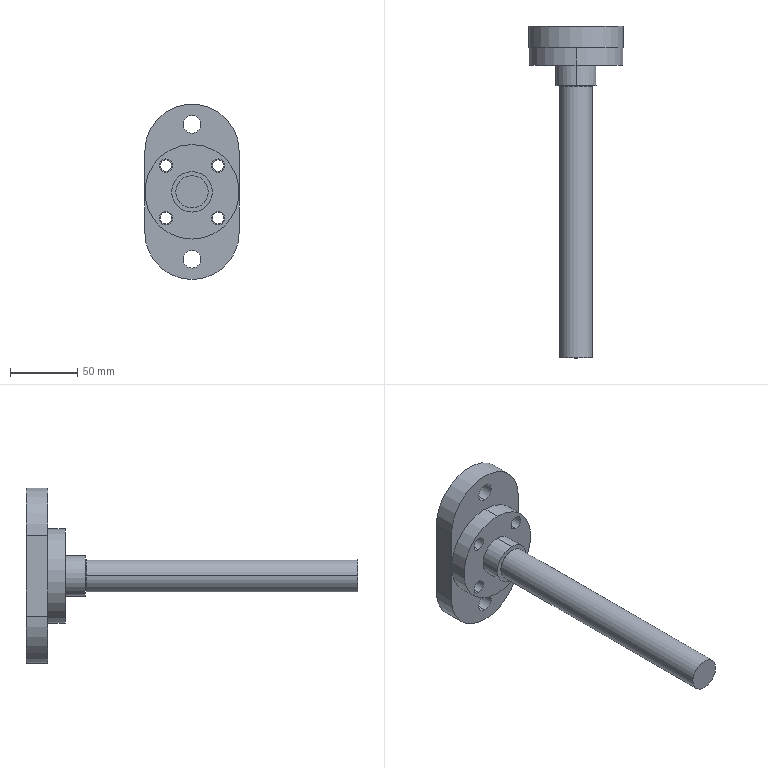Part | SolidWorks | features BaseBody 3 | 3 solids | 47 faces | box 70 x 246 x 130 mm | volume 268794 mm3 | cylinder 33 | plane 10 | cone 4 | commonest cylinder face diameters 8.5 x8 10 x8 70 x5 13 x4 16 x4 24 x2
STEP:
#1=CARTESIAN_POINT('',(-7.26,190.,0.));
#2=VERTEX_POINT('',#1);
#3=CARTESIAN_POINT('',(7.26,190.,0.));
#4=VERTEX_POINT('',#3);
#5=CARTESIAN_POINT('',(0.,190.,0.));
#6=DIRECTION('',(0.,1.,0.));
#7=DIRECTION('',(1.,0.,0.));
#8=AXIS2_PLACEMENT_3D('',#5,#6,#7);
#9=CIRCLE('',#8,7.26);
#10=EDGE_CURVE('',#2,#4,#9,.T.);
#11=ORIENTED_EDGE('',*,*,#10,.F.);
#12=CARTESIAN_POINT('',(-8.,189.26,0.));
#13=VERTEX_POINT('',#12);
#14=CARTESIAN_POINT('',(-7.26,190.,0.));
#15=DIRECTION('',(-0.7071,-0.7071,0.));
#16=VECTOR('',#15,1000.);
#17=LINE('',#14,#16);
#18=EDGE_CURVE('',#2,#13,#17,.T.);
#19=ORIENTED_EDGE('',*,*,#18,.T.);
#20=CARTESIAN_POINT('',(8.,189.26,0.));
#21=VERTEX_POINT('',#20);
#22=CARTESIAN_POINT('',(0.,189.26,0.));
#23=DIRECTION('',(0.,-1.,0.));
#24=DIRECTION('',(1.,0.,0.));
#25=AXIS2_PLACEMENT_3D('',#22,#23,#24);
#26=CIRCLE('',#25,8.);
#27=EDGE_CURVE('',#21,#13,#26,.T.);
#28=ORIENTED_EDGE('',*,*,#27,.F.);
#29=CARTESIAN_POINT('',(7.26,190.,0.));
#30=DIRECTION('',(0.7071,-0.7071,0.));
#31=VECTOR('',#30,1000.);
#32=LINE('',#29,#31);
#33=EDGE_CURVE('',#4,#21,#32,.T.);
#34=ORIENTED_EDGE('',*,*,#33,.F.);
#35=EDGE_LOOP('',(#11,#19,#28,#34));
#36=FACE_OUTER_BOUND('',#35,.T.);
#37=CARTESIAN_POINT('',(0.,190.,0.));
#38=DIRECTION('',(0.,-1.,0.));
#39=DIRECTION('',(1.,0.,0.));
#40=AXIS2_PLACEMENT_3D('',#37,#38,#39);
#41=CONICAL_SURFACE('',#40,7.26,0.7854);
#42=ADVANCED_FACE('',(#36),#41,.T.);
#43=CARTESIAN_POINT('',(-11.26,162.,0.));
#44=VERTEX_POINT('',#43);
#45=CARTESIAN_POINT('',(11.26,162.,0.));
#46=VERTEX_POINT('',#45);
#47=CARTESIAN_POINT('',(0.,162.,0.));
#48=DIRECTION('',(0.,1.,0.));
#49=DIRECTION('',(1.,0.,0.));
#50=AXIS2_PLACEMENT_3D('',#47,#48,#49);
#51=CIRCLE('',#50,11.26);
#52=EDGE_CURVE('',#44,#46,#51,.T.);
#53=ORIENTED_EDGE('',*,*,#52,.F.);
#54=CARTESIAN_POINT('',(-12.,161.26,0.));
#55=VERTEX_POINT('',#54);
#56=CARTESIAN_POINT('',(-11.26,162.,0.));
#57=DIRECTION('',(-0.7071,-0.7071,0.));
#58=VECTOR('',#57,1000.);
#59=LINE('',#56,#58);
#60=EDGE_CURVE('',#44,#55,#59,.T.);
#61=ORIENTED_EDGE('',*,*,#60,.T.);
#62=CARTESIAN_POINT('',(12.,161.26,0.));
#63=VERTEX_POINT('',#62);
#64=CARTESIAN_POINT('',(0.,161.26,0.));
#65=DIRECTION('',(0.,-1.,0.));
#66=DIRECTION('',(1.,0.,0.));
#67=AXIS2_PLACEMENT_3D('',#64,#65,#66);
#68=CIRCLE('',#67,12.);
#69=EDGE_CURVE('',#63,#55,#68,.T.);
#70=ORIENTED_EDGE('',*,*,#69,.F.);
#71=CARTESIAN_POINT('',(11.26,162.,0.));
#72=DIRECTION('',(0.7071,-0.7071,0.));
#73=VECTOR('',#72,1000.);
#74=LINE('',#71,#73);
#75=EDGE_CURVE('',#46,#63,#74,.T.);
#76=ORIENTED_EDGE('',*,*,#75,.F.);
#77=EDGE_LOOP('',(#53,#61,#70,#76));
#78=FACE_OUTER_BOUND('',#77,.T.);
#79=CARTESIAN_POINT('',(0.,162.,0.));
#80=DIRECTION('',(0.,-1.,0.));
#81=DIRECTION('',(1.,0.,0.));
#82=AXIS2_PLACEMENT_3D('',#79,#80,#81);
#83=CONICAL_SURFACE('',#82,11.26,0.7854);
#84=ADVANCED_FACE('',(#78),#83,.T.);
#85=CARTESIAN_POINT('',(-8.,162.,0.));
#86=VERTEX_POINT('',#85);
#87=CARTESIAN_POINT('',(8.,162.,0.));
#88=VERTEX_POINT('',#87);
#89=CARTESIAN_POINT('',(0.,162.,0.));
#90=DIRECTION('',(0.,1.,0.));
#91=DIRECTION('',(-1.,0.,0.));
#92=AXIS2_PLACEMENT_3D('',#89,#90,#91);
#93=CIRCLE('',#92,8.);
#94=EDGE_CURVE('',#86,#88,#93,.T.);
#95=ORIENTED_EDGE('',*,*,#94,.T.);
#96=CARTESIAN_POINT('',(8.,60.,0.));
#97=DIRECTION('',(0.,1.,0.));
#98=VECTOR('',#97,1000.);
#99=LINE('',#96,#98);
#100=EDGE_CURVE('',#88,#21,#99,.T.);
#101=ORIENTED_EDGE('',*,*,#100,.T.);
#102=ORIENTED_EDGE('',*,*,#27,.T.);
#103=CARTESIAN_POINT('',(-8.,60.,0.));
#104=DIRECTION('',(0.,1.,0.));
#105=VECTOR('',#104,1000.);
#106=LINE('',#103,#105);
#107=EDGE_CURVE('',#86,#13,#106,.T.);
#108=ORIENTED_EDGE('',*,*,#107,.F.);
#109=EDGE_LOOP('',(#95,#101,#102,#108));
#110=FACE_OUTER_BOUND('',#109,.T.);
#111=CARTESIAN_POINT('',(0.,60.,0.));
#112=DIRECTION('',(0.,1.,0.));
#113=DIRECTION('',(-1.,0.,0.));
#114=AXIS2_PLACEMENT_3D('',#111,#112,#113);
#115=CYLINDRICAL_SURFACE('',#114,8.);
#116=ADVANCED_FACE('',(#110),#115,.T.);
#117=CARTESIAN_POINT('',(-12.,-40.,0.));
#118=VERTEX_POINT('',#117);
#119=CARTESIAN_POINT('',(12.,-40.,0.));
#120=VERTEX_POINT('',#119);
#121=CARTESIAN_POINT('',(0.,-40.,0.));
#122=DIRECTION('',(0.,1.,0.));
#123=DIRECTION('',(-1.,0.,0.));
#124=AXIS2_PLACEMENT_3D('',#121,#122,#123);
#125=CIRCLE('',#124,12.);
#126=EDGE_CURVE('',#118,#120,#125,.T.);
#127=ORIENTED_EDGE('',*,*,#126,.T.);
#128=CARTESIAN_POINT('',(12.,60.,0.));
#129=DIRECTION('',(0.,1.,0.));
#130=VECTOR('',#129,1000.);
#131=LINE('',#128,#130);
#132=EDGE_CURVE('',#120,#63,#131,.T.);
#133=ORIENTED_EDGE('',*,*,#132,.T.);
#134=ORIENTED_EDGE('',*,*,#69,.T.);
#135=CARTESIAN_POINT('',(-12.,60.,0.));
#136=DIRECTION('',(0.,1.,0.));
#137=VECTOR('',#136,1000.);
#138=LINE('',#135,#137);
#139=EDGE_CURVE('',#118,#55,#138,.T.);
#140=ORIENTED_EDGE('',*,*,#139,.F.);
#141=EDGE_LOOP('',(#127,#133,#134,#140));
#142=FACE_OUTER_BOUND('',#141,.T.);
#143=CARTESIAN_POINT('',(0.,60.,0.));
#144=DIRECTION('',(0.,1.,0.));
#145=DIRECTION('',(-1.,0.,0.));
#146=AXIS2_PLACEMENT_3D('',#143,#144,#145);
#147=CYLINDRICAL_SURFACE('',#146,12.);
#148=ADVANCED_FACE('',(#142),#147,.T.);
#149=ORIENTED_EDGE('',*,*,#126,.F.);
#150=CARTESIAN_POINT('',(0.,-40.,0.));
#151=DIRECTION('',(0.,1.,0.));
#152=DIRECTION('',(-1.,0.,0.));
#153=AXIS2_PLACEMENT_3D('',#150,#151,#152);
#154=CIRCLE('',#153,12.);
#155=EDGE_CURVE('',#120,#118,#154,.T.);
#156=ORIENTED_EDGE('',*,*,#155,.F.);
#157=EDGE_LOOP('',(#149,#156));
#158=FACE_OUTER_BOUND('',#157,.T.);
#159=CARTESIAN_POINT('',(-12.,-40.,0.));
#160=DIRECTION('',(0.,1.,0.));
#161=DIRECTION('',(-1.,0.,0.));
#162=AXIS2_PLACEMENT_3D('',#159,#160,#161);
#163=PLANE('',#162);
#164=ADVANCED_FACE('',(#158),#163,.F.);
#165=ORIENTED_EDGE('',*,*,#132,.F.);
#166=ORIENTED_EDGE('',*,*,#155,.T.);
#167=ORIENTED_EDGE('',*,*,#139,.T.);
#168=CARTESIAN_POINT('',(0.,161.26,0.));
#169=DIRECTION('',(0.,-1.,0.));
#170=DIRECTION('',(1.,0.,0.));
#171=AXIS2_PLACEMENT_3D('',#168,#169,#170);
#172=CIRCLE('',#171,12.);
#173=EDGE_CURVE('',#55,#63,#172,.T.);
#174=ORIENTED_EDGE('',*,*,#173,.T.);
#175=EDGE_LOOP('',(#165,#166,#167,#174));
#176=FACE_OUTER_BOUND('',#175,.T.);
#177=CARTESIAN_POINT('',(0.,60.,0.));
#178=DIRECTION('',(0.,1.,0.));
#179=DIRECTION('',(-1.,0.,0.));
#180=AXIS2_PLACEMENT_3D('',#177,#178,#179);
#181=CYLINDRICAL_SURFACE('',#180,12.);
#182=ADVANCED_FACE('',(#176),#181,.T.);
#183=CARTESIAN_POINT('',(0.,162.,0.));
#184=DIRECTION('',(0.,1.,0.));
#185=DIRECTION('',(1.,0.,0.));
#186=AXIS2_PLACEMENT_3D('',#183,#184,#185);
#187=CIRCLE('',#186,11.26);
#188=EDGE_CURVE('',#46,#44,#187,.T.);
#189=ORIENTED_EDGE('',*,*,#188,.T.);
#190=ORIENTED_EDGE('',*,*,#52,.T.);
#191=EDGE_LOOP('',(#189,#190));
#192=FACE_OUTER_BOUND('',#191,.T.);
#193=ORIENTED_EDGE('',*,*,#94,.F.);
#194=CARTESIAN_POINT('',(0.,162.,0.));
#195=DIRECTION('',(0.,1.,0.));
#196=DIRECTION('',(-1.,0.,0.));
#197=AXIS2_PLACEMENT_3D('',#194,#195,#196);
#198=CIRCLE('',#197,8.);
#199=EDGE_CURVE('',#88,#86,#198,.T.);
#200=ORIENTED_EDGE('',*,*,#199,.F.);
#201=EDGE_LOOP('',(#193,#200));
#202=FACE_BOUND('',#201,.T.);
#203=CARTESIAN_POINT('',(-8.,162.,0.));
#204=DIRECTION('',(0.,-1.,0.));
#205=DIRECTION('',(1.,0.,0.));
#206=AXIS2_PLACEMENT_3D('',#203,#204,#205);
#207=PLANE('',#206);
#208=ADVANCED_FACE('',(#192,#202),#207,.F.);
#209=ORIENTED_EDGE('',*,*,#100,.F.);
#210=ORIENTED_EDGE('',*,*,#199,.T.);
#211=ORIENTED_EDGE('',*,*,#107,.T.);
#212=CARTESIAN_POINT('',(0.,189.26,0.));
#213=DIRECTION('',(0.,-1.,0.));
#214=DIRECTION('',(1.,0.,0.));
#215=AXIS2_PLACEMENT_3D('',#212,#213,#214);
#216=CIRCLE('',#215,8.);
#217=EDGE_CURVE('',#13,#21,#216,.T.);
#218=ORIENTED_EDGE('',*,*,#217,.T.);
#219=EDGE_LOOP('',(#209,#210,#211,#218));
#220=FACE_OUTER_BOUND('',#219,.T.);
#221=CARTESIAN_POINT('',(0.,60.,0.));
#222=DIRECTION('',(0.,1.,0.));
#223=DIRECTION('',(-1.,0.,0.));
#224=AXIS2_PLACEMENT_3D('',#221,#222,#223);
#225=CYLINDRICAL_SURFACE('',#224,8.);
#226=ADVANCED_FACE('',(#220),#225,.T.);
#227=CARTESIAN_POINT('',(0.,190.,0.));
#228=DIRECTION('',(0.,1.,0.));
#229=DIRECTION('',(1.,0.,0.));
#230=AXIS2_PLACEMENT_3D('',#227,#228,#229);
#231=CIRCLE('',#230,7.26);
#232=EDGE_CURVE('',#4,#2,#231,.T.);
#233=ORIENTED_EDGE('',*,*,#232,.T.);
#234=ORIENTED_EDGE('',*,*,#10,.T.);
#235=EDGE_LOOP('',(#233,#234));
#236=FACE_OUTER_BOUND('',#235,.T.);
#237=CARTESIAN_POINT('',(0.,190.,0.));
#238=DIRECTION('',(0.,-1.,0.));
#239=DIRECTION('',(1.,0.,0.));
#240=AXIS2_PLACEMENT_3D('',#237,#238,#239);
#241=PLANE('',#240);
#242=ADVANCED_FACE('',(#236),#241,.F.);
#243=ORIENTED_EDGE('',*,*,#60,.F.);
#244=ORIENTED_EDGE('',*,*,#188,.F.);
#245=ORIENTED_EDGE('',*,*,#75,.T.);
#246=ORIENTED_EDGE('',*,*,#173,.F.);
#247=EDGE_LOOP('',(#243,#244,#245,#246));
#248=FACE_OUTER_BOUND('',#247,.T.);
#249=CARTESIAN_POINT('',(0.,162.,0.));
#250=DIRECTION('',(0.,-1.,0.));
#251=DIRECTION('',(1.,0.,0.));
#252=AXIS2_PLACEMENT_3D('',#249,#250,#251);
#253=CONICAL_SURFACE('',#252,11.26,0.7854);
#254=ADVANCED_FACE('',(#248),#253,.T.);
#255=ORIENTED_EDGE('',*,*,#18,.F.);
#256=ORIENTED_EDGE('',*,*,#232,.F.);
#257=ORIENTED_EDGE('',*,*,#33,.T.);
#258=ORIENTED_EDGE('',*,*,#217,.F.);
#259=EDGE_LOOP('',(#255,#256,#257,#258));
#260=FACE_OUTER_BOUND('',#259,.T.);
#261=CARTESIAN_POINT('',(0.,190.,0.));
#262=DIRECTION('',(0.,-1.,0.));
#263=DIRECTION('',(1.,0.,0.));
#264=AXIS2_PLACEMENT_3D('',#261,#262,#263);
#265=CONICAL_SURFACE('',#264,7.26,0.7854);
#266=ADVANCED_FACE('',(#260),#265,.T.);
#267=CLOSED_SHELL('',(#42,#84,#116,#148,#164,#182,#208,#226,#242,#254,#266));
#268=MANIFOLD_SOLID_BREP('',#267);
#269=CARTESIAN_POINT('',(19.445,190.,-14.445));
#270=VERTEX_POINT('',#269);
#271=CARTESIAN_POINT('',(19.445,190.,-24.445));
#272=VERTEX_POINT('',#271);
#273=CARTESIAN_POINT('',(19.445,190.,-19.445));
#274=DIRECTION('',(0.,-1.,0.));
#275=DIRECTION('',(0.,0.,-1.));
#276=AXIS2_PLACEMENT_3D('',#273,#274,#275);
#277=CIRCLE('',#276,5.);
#278=EDGE_CURVE('',#270,#272,#277,.T.);
#279=ORIENTED_EDGE('',*,*,#278,.F.);
#280=CARTESIAN_POINT('',(19.445,177.,-14.445));
#281=VERTEX_POINT('',#280);
#282=CARTESIAN_POINT('',(19.445,177.,-14.445));
#283=DIRECTION('',(0.,-1.,0.));
#284=VECTOR('',#283,1000.);
#285=LINE('',#282,#284);
#286=EDGE_CURVE('',#270,#281,#285,.T.);
#287=ORIENTED_EDGE('',*,*,#286,.T.);
#288=CARTESIAN_POINT('',(19.445,177.,-24.445));
#289=VERTEX_POINT('',#288);
#290=CARTESIAN_POINT('',(19.445,177.,-19.445));
#291=DIRECTION('',(0.,-1.,0.));
#292=DIRECTION('',(0.,0.,-1.));
#293=AXIS2_PLACEMENT_3D('',#290,#291,#292);
#294=CIRCLE('',#293,5.);
#295=EDGE_CURVE('',#281,#289,#294,.T.);
#296=ORIENTED_EDGE('',*,*,#295,.T.);
#297=CARTESIAN_POINT('',(19.445,177.,-24.445));
#298=DIRECTION('',(0.,-1.,0.));
#299=VECTOR('',#298,1000.);
#300=LINE('',#297,#299);
#301=EDGE_CURVE('',#272,#289,#300,.T.);
#302=ORIENTED_EDGE('',*,*,#301,.F.);
#303=EDGE_LOOP('',(#279,#287,#296,#302));
#304=FACE_OUTER_BOUND('',#303,.T.);
#305=CARTESIAN_POINT('',(19.445,177.,-19.445));
#306=DIRECTION('',(0.,-1.,0.));
#307=DIRECTION('',(0.,0.,-1.));
#308=AXIS2_PLACEMENT_3D('',#305,#306,#307);
#309=CYLINDRICAL_SURFACE('',#308,5.);
#310=ADVANCED_FACE('',(#304),#309,.F.);
#311=CARTESIAN_POINT('',(-19.445,190.,-14.445));
#312=VERTEX_POINT('',#311);
#313=CARTESIAN_POINT('',(-19.445,190.,-24.445));
#314=VERTEX_POINT('',#313);
#315=CARTESIAN_POINT('',(-19.445,190.,-19.445));
#316=DIRECTION('',(0.,-1.,0.));
#317=DIRECTION('',(0.,0.,-1.));
#318=AXIS2_PLACEMENT_3D('',#315,#316,#317);
#319=CIRCLE('',#318,5.);
#320=EDGE_CURVE('',#312,#314,#319,.T.);
#321=ORIENTED_EDGE('',*,*,#320,.F.);
#322=CARTESIAN_POINT('',(-19.445,177.,-14.445));
#323=VERTEX_POINT('',#322);
#324=CARTESIAN_POINT('',(-19.445,177.,-14.445));
#325=DIRECTION('',(0.,-1.,0.));
#326=VECTOR('',#325,1000.);
#327=LINE('',#324,#326);
#328=EDGE_CURVE('',#312,#323,#327,.T.);
#329=ORIENTED_EDGE('',*,*,#328,.T.);
#330=CARTESIAN_POINT('',(-19.445,177.,-24.445));
#331=VERTEX_POINT('',#330);
#332=CARTESIAN_POINT('',(-19.445,177.,-19.445));
#333=DIRECTION('',(0.,-1.,0.));
#334=DIRECTION('',(0.,0.,-1.));
#335=AXIS2_PLACEMENT_3D('',#332,#333,#334);
#336=CIRCLE('',#335,5.);
#337=EDGE_CURVE('',#323,#331,#336,.T.);
#338=ORIENTED_EDGE('',*,*,#337,.T.);
#339=CARTESIAN_POINT('',(-19.445,177.,-24.445));
#340=DIRECTION('',(0.,-1.,0.));
#341=VECTOR('',#340,1000.);
#342=LINE('',#339,#341);
#343=EDGE_CURVE('',#314,#331,#342,.T.);
#344=ORIENTED_EDGE('',*,*,#343,.F.);
#345=EDGE_LOOP('',(#321,#329,#338,#344));
#346=FACE_OUTER_BOUND('',#345,.T.);
#347=CARTESIAN_POINT('',(-19.445,177.,-19.445));
#348=DIRECTION('',(0.,-1.,0.));
#349=DIRECTION('',(0.,0.,-1.));
#350=AXIS2_PLACEMENT_3D('',#347,#348,#349);
#351=CYLINDRICAL_SURFACE('',#350,5.);
#352=ADVANCED_FACE('',(#346),#351,.F.);
#353=CARTESIAN_POINT('',(-19.445,190.,24.445));
#354=VERTEX_POINT('',#353);
#355=CARTESIAN_POINT('',(-19.445,190.,14.445));
#356=VERTEX_POINT('',#355);
#357=CARTESIAN_POINT('',(-19.445,190.,19.445));
#358=DIRECTION('',(0.,-1.,0.));
#359=DIRECTION('',(0.,0.,-1.));
#360=AXIS2_PLACEMENT_3D('',#357,#358,#359);
#361=CIRCLE('',#360,5.);
#362=EDGE_CURVE('',#354,#356,#361,.T.);
#363=ORIENTED_EDGE('',*,*,#362,.F.);
#364=CARTESIAN_POINT('',(-19.445,177.,24.445));
#365=VERTEX_POINT('',#364);
#366=CARTESIAN_POINT('',(-19.445,177.,24.445));
#367=DIRECTION('',(0.,-1.,0.));
#368=VECTOR('',#367,1000.);
#369=LINE('',#366,#368);
#370=EDGE_CURVE('',#354,#365,#369,.T.);
#371=ORIENTED_EDGE('',*,*,#370,.T.);
#372=CARTESIAN_POINT('',(-19.445,177.,14.445));
#373=VERTEX_POINT('',#372);
#374=CARTESIAN_POINT('',(-19.445,177.,19.445));
#375=DIRECTION('',(0.,-1.,0.));
#376=DIRECTION('',(0.,0.,-1.));
#377=AXIS2_PLACEMENT_3D('',#374,#375,#376);
#378=CIRCLE('',#377,5.);
#379=EDGE_CURVE('',#365,#373,#378,.T.);
#380=ORIENTED_EDGE('',*,*,#379,.T.);
#381=CARTESIAN_POINT('',(-19.445,177.,14.445));
#382=DIRECTION('',(0.,-1.,0.));
#383=VECTOR('',#382,1000.);
#384=LINE('',#381,#383);
#385=EDGE_CURVE('',#356,#373,#384,.T.);
#386=ORIENTED_EDGE('',*,*,#385,.F.);
#387=EDGE_LOOP('',(#363,#371,#380,#386));
#388=FACE_OUTER_BOUND('',#387,.T.);
#389=CARTESIAN_POINT('',(-19.445,177.,19.445));
#390=DIRECTION('',(0.,-1.,0.));
#391=DIRECTION('',(0.,0.,-1.));
#392=AXIS2_PLACEMENT_3D('',#389,#390,#391);
#393=CYLINDRICAL_SURFACE('',#392,5.);
#394=ADVANCED_FACE('',(#388),#393,.F.);
#395=CARTESIAN_POINT('',(19.445,190.,24.445));
#396=VERTEX_POINT('',#395);
#397=CARTESIAN_POINT('',(19.445,190.,14.445));
#398=VERTEX_POINT('',#397);
#399=CARTESIAN_POINT('',(19.445,190.,19.445));
#400=DIRECTION('',(0.,-1.,0.));
#401=DIRECTION('',(0.,0.,-1.));
#402=AXIS2_PLACEMENT_3D('',#399,#400,#401);
#403=CIRCLE('',#402,5.);
#404=EDGE_CURVE('',#396,#398,#403,.T.);
#405=ORIENTED_EDGE('',*,*,#404,.F.);
#406=CARTESIAN_POINT('',(19.445,177.,24.445));
#407=VERTEX_POINT('',#406);
#408=CARTESIAN_POINT('',(19.445,177.,24.445));
#409=DIRECTION('',(0.,-1.,0.));
#410=VECTOR('',#409,1000.);
#411=LINE('',#408,#410);
#412=EDGE_CURVE('',#396,#407,#411,.T.);
#413=ORIENTED_EDGE('',*,*,#412,.T.);
#414=CARTESIAN_POINT('',(19.445,177.,14.445));
#415=VERTEX_POINT('',#414);
#416=CARTESIAN_POINT('',(19.445,177.,19.445));
#417=DIRECTION('',(0.,-1.,0.));
#418=DIRECTION('',(0.,0.,-1.));
#419=AXIS2_PLACEMENT_3D('',#416,#417,#418);
#420=CIRCLE('',#419,5.);
#421=EDGE_CURVE('',#407,#415,#420,.T.);
#422=ORIENTED_EDGE('',*,*,#421,.T.);
#423=CARTESIAN_POINT('',(19.445,177.,14.445));
#424=DIRECTION('',(0.,-1.,0.));
#425=VECTOR('',#424,1000.);
#426=LINE('',#423,#425);
#427=EDGE_CURVE('',#398,#415,#426,.T.);
#428=ORIENTED_EDGE('',*,*,#427,.F.);
#429=EDGE_LOOP('',(#405,#413,#422,#428));
#430=FACE_OUTER_BOUND('',#429,.T.);
#431=CARTESIAN_POINT('',(19.445,177.,19.445));
#432=DIRECTION('',(0.,-1.,0.));
#433=DIRECTION('',(0.,0.,-1.));
#434=AXIS2_PLACEMENT_3D('',#431,#432,#433);
#435=CYLINDRICAL_SURFACE('',#434,5.);
#436=ADVANCED_FACE('',(#430),#435,.F.);
#437=CARTESIAN_POINT('',(0.,177.,35.));
#438=VERTEX_POINT('',#437);
#439=CARTESIAN_POINT('',(0.,177.,-35.));
#440=VERTEX_POINT('',#439);
#441=CARTESIAN_POINT('',(0.,177.,0.));
#442=DIRECTION('',(0.,1.,0.));
#443=DIRECTION('',(0.,0.,1.));
#444=AXIS2_PLACEMENT_3D('',#441,#442,#443);
#445=CIRCLE('',#444,35.);
#446=EDGE_CURVE('',#438,#440,#445,.T.);
#447=ORIENTED_EDGE('',*,*,#446,.T.);
#448=CARTESIAN_POINT('',(0.,190.,-35.));
#449=VERTEX_POINT('',#448);
#450=CARTESIAN_POINT('',(0.,190.,-35.));
#451=DIRECTION('',(0.,1.,0.));
#452=VECTOR('',#451,1000.);
#453=LINE('',#450,#452);
#454=EDGE_CURVE('',#440,#449,#453,.T.);
#455=ORIENTED_EDGE('',*,*,#454,.T.);
#456=CARTESIAN_POINT('',(0.,190.,35.));
#457=VERTEX_POINT('',#456);
#458=CARTESIAN_POINT('',(0.,190.,0.));
#459=DIRECTION('',(0.,1.,0.));
#460=DIRECTION('',(0.,0.,1.));
#461=AXIS2_PLACEMENT_3D('',#458,#459,#460);
#462=CIRCLE('',#461,35.);
#463=EDGE_CURVE('',#457,#449,#462,.T.);
#464=ORIENTED_EDGE('',*,*,#463,.F.);
#465=CARTESIAN_POINT('',(0.,190.,35.));
#466=DIRECTION('',(0.,1.,0.));
#467=VECTOR('',#466,1000.);
#468=LINE('',#465,#467);
#469=EDGE_CURVE('',#438,#457,#468,.T.);
#470=ORIENTED_EDGE('',*,*,#469,.F.);
#471=EDGE_LOOP('',(#447,#455,#464,#470));
#472=FACE_OUTER_BOUND('',#471,.T.);
#473=CARTESIAN_POINT('',(0.,190.,0.));
#474=DIRECTION('',(0.,1.,0.));
#475=DIRECTION('',(0.,0.,1.));
#476=AXIS2_PLACEMENT_3D('',#473,#474,#475);
#477=CYLINDRICAL_SURFACE('',#476,35.);
#478=ADVANCED_FACE('',(#472),#477,.T.);
#479=CARTESIAN_POINT('',(0.,162.,15.));
#480=VERTEX_POINT('',#479);
#481=CARTESIAN_POINT('',(0.,162.,-15.));
#482=VERTEX_POINT('',#481);
#483=CARTESIAN_POINT('',(0.,162.,0.));
#484=DIRECTION('',(0.,1.,0.));
#485=DIRECTION('',(0.,0.,1.));
#486=AXIS2_PLACEMENT_3D('',#483,#484,#485);
#487=CIRCLE('',#486,15.);
#488=EDGE_CURVE('',#480,#482,#487,.T.);
#489=ORIENTED_EDGE('',*,*,#488,.T.);
#490=CARTESIAN_POINT('',(0.,177.,-15.));
#491=VERTEX_POINT('',#490);
#492=CARTESIAN_POINT('',(0.,190.,-15.));
#493=DIRECTION('',(0.,1.,0.));
#494=VECTOR('',#493,1000.);
#495=LINE('',#492,#494);
#496=EDGE_CURVE('',#482,#491,#495,.T.);
#497=ORIENTED_EDGE('',*,*,#496,.T.);
#498=CARTESIAN_POINT('',(0.,177.,15.));
#499=VERTEX_POINT('',#498);
#500=CARTESIAN_POINT('',(0.,177.,0.));
#501=DIRECTION('',(0.,1.,0.));
#502=DIRECTION('',(0.,0.,1.));
#503=AXIS2_PLACEMENT_3D('',#500,#501,#502);
#504=CIRCLE('',#503,15.);
#505=EDGE_CURVE('',#499,#491,#504,.T.);
#506=ORIENTED_EDGE('',*,*,#505,.F.);
#507=CARTESIAN_POINT('',(0.,190.,15.));
#508=DIRECTION('',(0.,1.,0.));
#509=VECTOR('',#508,1000.);
#510=LINE('',#507,#509);
#511=EDGE_CURVE('',#480,#499,#510,.T.);
#512=ORIENTED_EDGE('',*,*,#511,.F.);
#513=EDGE_LOOP('',(#489,#497,#506,#512));
#514=FACE_OUTER_BOUND('',#513,.T.);
#515=CARTESIAN_POINT('',(0.,190.,0.));
#516=DIRECTION('',(0.,1.,0.));
#517=DIRECTION('',(0.,0.,1.));
#518=AXIS2_PLACEMENT_3D('',#515,#516,#517);
#519=CYLINDRICAL_SURFACE('',#518,15.);
#520=ADVANCED_FACE('',(#514),#519,.T.);
#521=CARTESIAN_POINT('',(0.,162.,-8.));
#522=VERTEX_POINT('',#521);
#523=CARTESIAN_POINT('',(0.,162.,8.));
#524=VERTEX_POINT('',#523);
#525=CARTESIAN_POINT('',(0.,162.,0.));
#526=DIRECTION('',(0.,1.,0.));
#527=DIRECTION('',(0.,0.,1.));
#528=AXIS2_PLACEMENT_3D('',#525,#526,#527);
#529=CIRCLE('',#528,8.);
#530=EDGE_CURVE('',#522,#524,#529,.T.);
#531=ORIENTED_EDGE('',*,*,#530,.F.);
#532=CARTESIAN_POINT('',(0.,190.,-8.));
#533=VERTEX_POINT('',#532);
#534=CARTESIAN_POINT('',(0.,190.,-8.));
#535=DIRECTION('',(0.,1.,0.));
#536=VECTOR('',#535,1000.);
#537=LINE('',#534,#536);
#538=EDGE_CURVE('',#522,#533,#537,.T.);
#539=ORIENTED_EDGE('',*,*,#538,.T.);
#540=CARTESIAN_POINT('',(0.,190.,8.));
#541=VERTEX_POINT('',#540);
#542=CARTESIAN_POINT('',(0.,190.,0.));
#543=DIRECTION('',(0.,1.,0.));
#544=DIRECTION('',(0.,0.,1.));
#545=AXIS2_PLACEMENT_3D('',#542,#543,#544);
#546=CIRCLE('',#545,8.);
#547=EDGE_CURVE('',#533,#541,#546,.T.);
#548=ORIENTED_EDGE('',*,*,#547,.T.);
#549=CARTESIAN_POINT('',(0.,190.,8.));
#550=DIRECTION('',(0.,1.,0.));
#551=VECTOR('',#550,1000.);
#552=LINE('',#549,#551);
#553=EDGE_CURVE('',#524,#541,#552,.T.);
#554=ORIENTED_EDGE('',*,*,#553,.F.);
#555=EDGE_LOOP('',(#531,#539,#548,#554));
#556=FACE_OUTER_BOUND('',#555,.T.);
#557=CARTESIAN_POINT('',(0.,190.,0.));
#558=DIRECTION('',(0.,1.,0.));
#559=DIRECTION('',(0.,0.,1.));
#560=AXIS2_PLACEMENT_3D('',#557,#558,#559);
#561=CYLINDRICAL_SURFACE('',#560,8.);
#562=ADVANCED_FACE('',(#556),#561,.F.);
#563=ORIENTED_EDGE('',*,*,#538,.F.);
#564=CARTESIAN_POINT('',(0.,162.,0.));
#565=DIRECTION('',(0.,1.,0.));
#566=DIRECTION('',(0.,0.,1.));
#567=AXIS2_PLACEMENT_3D('',#564,#565,#566);
#568=CIRCLE('',#567,8.);
#569=EDGE_CURVE('',#524,#522,#568,.T.);
#570=ORIENTED_EDGE('',*,*,#569,.F.);
#571=ORIENTED_EDGE('',*,*,#553,.T.);
#572=CARTESIAN_POINT('',(0.,190.,0.));
#573=DIRECTION('',(0.,1.,0.));
#574=DIRECTION('',(0.,0.,1.));
#575=AXIS2_PLACEMENT_3D('',#572,#573,#574);
#576=CIRCLE('',#575,8.);
#577=EDGE_CURVE('',#541,#533,#576,.T.);
#578=ORIENTED_EDGE('',*,*,#577,.T.);
#579=EDGE_LOOP('',(#563,#570,#571,#578));
#580=FACE_OUTER_BOUND('',#579,.T.);
#581=CARTESIAN_POINT('',(0.,190.,0.));
#582=DIRECTION('',(0.,1.,0.));
#583=DIRECTION('',(0.,0.,1.));
#584=AXIS2_PLACEMENT_3D('',#581,#582,#583);
#585=CYLINDRICAL_SURFACE('',#584,8.);
#586=ADVANCED_FACE('',(#580),#585,.F.);
#587=ORIENTED_EDGE('',*,*,#488,.F.);
#588=CARTESIAN_POINT('',(0.,162.,0.));
#589=DIRECTION('',(0.,1.,0.));
#590=DIRECTION('',(0.,0.,1.));
#591=AXIS2_PLACEMENT_3D('',#588,#589,#590);
#592=CIRCLE('',#591,15.);
#593=EDGE_CURVE('',#482,#480,#592,.T.);
#594=ORIENTED_EDGE('',*,*,#593,.F.);
#595=EDGE_LOOP('',(#587,#594));
#596=FACE_OUTER_BOUND('',#595,.T.);
#597=ORIENTED_EDGE('',*,*,#569,.T.);
#598=ORIENTED_EDGE('',*,*,#530,.T.);
#599=EDGE_LOOP('',(#597,#598));
#600=FACE_BOUND('',#599,.T.);
#601=CARTESIAN_POINT('',(0.,162.,-8.));
#602=DIRECTION('',(0.,1.,0.));
#603=DIRECTION('',(0.,0.,1.));
#604=AXIS2_PLACEMENT_3D('',#601,#602,#603);
#605=PLANE('',#604);
#606=ADVANCED_FACE('',(#596,#600),#605,.F.);
#607=ORIENTED_EDGE('',*,*,#496,.F.);
#608=ORIENTED_EDGE('',*,*,#593,.T.);
#609=ORIENTED_EDGE('',*,*,#511,.T.);
#610=CARTESIAN_POINT('',(0.,177.,0.));
#611=DIRECTION('',(0.,1.,0.));
#612=DIRECTION('',(0.,0.,1.));
#613=AXIS2_PLACEMENT_3D('',#610,#611,#612);
#614=CIRCLE('',#613,15.);
#615=EDGE_CURVE('',#491,#499,#614,.T.);
#616=ORIENTED_EDGE('',*,*,#615,.F.);
#617=EDGE_LOOP('',(#607,#608,#609,#616));
#618=FACE_OUTER_BOUND('',#617,.T.);
#619=CARTESIAN_POINT('',(0.,190.,0.));
#620=DIRECTION('',(0.,1.,0.));
#621=DIRECTION('',(0.,0.,1.));
#622=AXIS2_PLACEMENT_3D('',#619,#620,#621);
#623=CYLINDRICAL_SURFACE('',#622,15.);
#624=ADVANCED_FACE('',(#618),#623,.T.);
#625=CARTESIAN_POINT('',(19.445,177.,-19.445));
#626=DIRECTION('',(0.,-1.,0.));
#627=DIRECTION('',(0.,0.,-1.));
#628=AXIS2_PLACEMENT_3D('',#625,#626,#627);
#629=CIRCLE('',#628,5.);
#630=EDGE_CURVE('',#289,#281,#629,.T.);
#631=ORIENTED_EDGE('',*,*,#630,.F.);
#632=ORIENTED_EDGE('',*,*,#295,.F.);
#633=EDGE_LOOP('',(#631,#632));
#634=FACE_BOUND('',#633,.T.);
#635=CARTESIAN_POINT('',(-19.445,177.,-19.445));
#636=DIRECTION('',(0.,-1.,0.));
#637=DIRECTION('',(0.,0.,-1.));
#638=AXIS2_PLACEMENT_3D('',#635,#636,#637);
#639=CIRCLE('',#638,5.);
#640=EDGE_CURVE('',#331,#323,#639,.T.);
#641=ORIENTED_EDGE('',*,*,#640,.F.);
#642=ORIENTED_EDGE('',*,*,#337,.F.);
#643=EDGE_LOOP('',(#641,#642));
#644=FACE_BOUND('',#643,.T.);
#645=CARTESIAN_POINT('',(-19.445,177.,19.445));
#646=DIRECTION('',(0.,-1.,0.));
#647=DIRECTION('',(0.,0.,-1.));
#648=AXIS2_PLACEMENT_3D('',#645,#646,#647);
#649=CIRCLE('',#648,5.);
#650=EDGE_CURVE('',#373,#365,#649,.T.);
#651=ORIENTED_EDGE('',*,*,#650,.F.);
#652=ORIENTED_EDGE('',*,*,#379,.F.);
#653=EDGE_LOOP('',(#651,#652));
#654=FACE_BOUND('',#653,.T.);
#655=CARTESIAN_POINT('',(19.445,177.,19.445));
#656=DIRECTION('',(0.,-1.,0.));
#657=DIRECTION('',(0.,0.,-1.));
#658=AXIS2_PLACEMENT_3D('',#655,#656,#657);
#659=CIRCLE('',#658,5.);
#660=EDGE_CURVE('',#415,#407,#659,.T.);
#661=ORIENTED_EDGE('',*,*,#660,.F.);
#662=ORIENTED_EDGE('',*,*,#421,.F.);
#663=EDGE_LOOP('',(#661,#662));
#664=FACE_BOUND('',#663,.T.);
#665=ORIENTED_EDGE('',*,*,#446,.F.);
#666=CARTESIAN_POINT('',(0.,177.,0.));
#667=DIRECTION('',(0.,1.,0.));
#668=DIRECTION('',(0.,0.,1.));
#669=AXIS2_PLACEMENT_3D('',#666,#667,#668);
#670=CIRCLE('',#669,35.);
#671=EDGE_CURVE('',#440,#438,#670,.T.);
#672=ORIENTED_EDGE('',*,*,#671,.F.);
#673=EDGE_LOOP('',(#665,#672));
#674=FACE_OUTER_BOUND('',#673,.T.);
#675=ORIENTED_EDGE('',*,*,#505,.T.);
#676=ORIENTED_EDGE('',*,*,#615,.T.);
#677=EDGE_LOOP('',(#675,#676));
#678=FACE_BOUND('',#677,.T.);
#679=CARTESIAN_POINT('',(0.,177.,-15.));
#680=DIRECTION('',(0.,1.,0.));
#681=DIRECTION('',(0.,0.,1.));
#682=AXIS2_PLACEMENT_3D('',#679,#680,#681);
#683=PLANE('',#682);
#684=ADVANCED_FACE('',(#634,#644,#654,#664,#674,#678),#683,.F.);
#685=ORIENTED_EDGE('',*,*,#454,.F.);
#686=ORIENTED_EDGE('',*,*,#671,.T.);
#687=ORIENTED_EDGE('',*,*,#469,.T.);
#688=CARTESIAN_POINT('',(0.,190.,0.));
#689=DIRECTION('',(0.,1.,0.));
#690=DIRECTION('',(0.,0.,1.));
#691=AXIS2_PLACEMENT_3D('',#688,#689,#690);
#692=CIRCLE('',#691,35.);
#693=EDGE_CURVE('',#449,#457,#692,.T.);
#694=ORIENTED_EDGE('',*,*,#693,.F.);
#695=EDGE_LOOP('',(#685,#686,#687,#694));
#696=FACE_OUTER_BOUND('',#695,.T.);
#697=CARTESIAN_POINT('',(0.,190.,0.));
#698=DIRECTION('',(0.,1.,0.));
#699=DIRECTION('',(0.,0.,1.));
#700=AXIS2_PLACEMENT_3D('',#697,#698,#699);
#701=CYLINDRICAL_SURFACE('',#700,35.);
#702=ADVANCED_FACE('',(#696),#701,.T.);
#703=CARTESIAN_POINT('',(19.445,190.,-19.445));
#704=DIRECTION('',(0.,-1.,0.));
#705=DIRECTION('',(0.,0.,-1.));
#706=AXIS2_PLACEMENT_3D('',#703,#704,#705);
#707=CIRCLE('',#706,5.);
#708=EDGE_CURVE('',#272,#270,#707,.T.);
#709=ORIENTED_EDGE('',*,*,#708,.T.);
#710=ORIENTED_EDGE('',*,*,#278,.T.);
#711=EDGE_LOOP('',(#709,#710));
#712=FACE_BOUND('',#711,.T.);
#713=CARTESIAN_POINT('',(-19.445,190.,-19.445));
#714=DIRECTION('',(0.,-1.,0.));
#715=DIRECTION('',(0.,0.,-1.));
#716=AXIS2_PLACEMENT_3D('',#713,#714,#715);
#717=CIRCLE('',#716,5.);
#718=EDGE_CURVE('',#314,#312,#717,.T.);
#719=ORIENTED_EDGE('',*,*,#718,.T.);
#720=ORIENTED_EDGE('',*,*,#320,.T.);
#721=EDGE_LOOP('',(#719,#720));
#722=FACE_BOUND('',#721,.T.);
#723=CARTESIAN_POINT('',(-19.445,190.,19.445));
#724=DIRECTION('',(0.,-1.,0.));
#725=DIRECTION('',(0.,0.,-1.));
#726=AXIS2_PLACEMENT_3D('',#723,#724,#725);
#727=CIRCLE('',#726,5.);
#728=EDGE_CURVE('',#356,#354,#727,.T.);
#729=ORIENTED_EDGE('',*,*,#728,.T.);
#730=ORIENTED_EDGE('',*,*,#362,.T.);
#731=EDGE_LOOP('',(#729,#730));
#732=FACE_BOUND('',#731,.T.);
#733=CARTESIAN_POINT('',(19.445,190.,19.445));
#734=DIRECTION('',(0.,-1.,0.));
#735=DIRECTION('',(0.,0.,-1.));
#736=AXIS2_PLACEMENT_3D('',#733,#734,#735);
#737=CIRCLE('',#736,5.);
#738=EDGE_CURVE('',#398,#396,#737,.T.);
#739=ORIENTED_EDGE('',*,*,#738,.T.);
#740=ORIENTED_EDGE('',*,*,#404,.T.);
#741=EDGE_LOOP('',(#739,#740));
#742=FACE_BOUND('',#741,.T.);
#743=ORIENTED_EDGE('',*,*,#577,.F.);
#744=ORIENTED_EDGE('',*,*,#547,.F.);
#745=EDGE_LOOP('',(#743,#744));
#746=FACE_BOUND('',#745,.T.);
#747=ORIENTED_EDGE('',*,*,#463,.T.);
#748=ORIENTED_EDGE('',*,*,#693,.T.);
#749=EDGE_LOOP('',(#747,#748));
#750=FACE_OUTER_BOUND('',#749,.T.);
#751=CARTESIAN_POINT('',(0.,190.,-35.));
#752=DIRECTION('',(0.,-1.,0.));
#753=DIRECTION('',(0.,0.,-1.));
#754=AXIS2_PLACEMENT_3D('',#751,#752,#753);
#755=PLANE('',#754);
#756=ADVANCED_FACE('',(#712,#722,#732,#742,#746,#750),#755,.F.);
#757=ORIENTED_EDGE('',*,*,#412,.F.);
#758=ORIENTED_EDGE('',*,*,#738,.F.);
#759=ORIENTED_EDGE('',*,*,#427,.T.);
#760=ORIENTED_EDGE('',*,*,#660,.T.);
#761=EDGE_LOOP('',(#757,#758,#759,#760));
#762=FACE_OUTER_BOUND('',#761,.T.);
#763=CARTESIAN_POINT('',(19.445,177.,19.445));
#764=DIRECTION('',(0.,-1.,0.));
#765=DIRECTION('',(0.,0.,-1.));
#766=AXIS2_PLACEMENT_3D('',#763,#764,#765);
#767=CYLINDRICAL_SURFACE('',#766,5.);
#768=ADVANCED_FACE('',(#762),#767,.F.);
#769=ORIENTED_EDGE('',*,*,#370,.F.);
#770=ORIENTED_EDGE('',*,*,#728,.F.);
#771=ORIENTED_EDGE('',*,*,#385,.T.);
#772=ORIENTED_EDGE('',*,*,#650,.T.);
#773=EDGE_LOOP('',(#769,#770,#771,#772));
#774=FACE_OUTER_BOUND('',#773,.T.);
#775=CARTESIAN_POINT('',(-19.445,177.,19.445));
#776=DIRECTION('',(0.,-1.,0.));
#777=DIRECTION('',(0.,0.,-1.));
#778=AXIS2_PLACEMENT_3D('',#775,#776,#777);
#779=CYLINDRICAL_SURFACE('',#778,5.);
#780=ADVANCED_FACE('',(#774),#779,.F.);
#781=ORIENTED_EDGE('',*,*,#328,.F.);
#782=ORIENTED_EDGE('',*,*,#718,.F.);
#783=ORIENTED_EDGE('',*,*,#343,.T.);
#784=ORIENTED_EDGE('',*,*,#640,.T.);
#785=EDGE_LOOP('',(#781,#782,#783,#784));
#786=FACE_OUTER_BOUND('',#785,.T.);
#787=CARTESIAN_POINT('',(-19.445,177.,-19.445));
#788=DIRECTION('',(0.,-1.,0.));
#789=DIRECTION('',(0.,0.,-1.));
#790=AXIS2_PLACEMENT_3D('',#787,#788,#789);
#791=CYLINDRICAL_SURFACE('',#790,5.);
#792=ADVANCED_FACE('',(#786),#791,.F.);
#793=ORIENTED_EDGE('',*,*,#286,.F.);
#794=ORIENTED_EDGE('',*,*,#708,.F.);
#795=ORIENTED_EDGE('',*,*,#301,.T.);
#796=ORIENTED_EDGE('',*,*,#630,.T.);
#797=EDGE_LOOP('',(#793,#794,#795,#796));
#798=FACE_OUTER_BOUND('',#797,.T.);
#799=CARTESIAN_POINT('',(19.445,177.,-19.445));
#800=DIRECTION('',(0.,-1.,0.));
#801=DIRECTION('',(0.,0.,-1.));
#802=AXIS2_PLACEMENT_3D('',#799,#800,#801);
#803=CYLINDRICAL_SURFACE('',#802,5.);
#804=ADVANCED_FACE('',(#798),#803,.F.);
#805=CLOSED_SHELL('',(#310,#352,#394,#436,#478,#520,#562,#586,#606,#624,#684,#702,#756,#768,#780,#792,#804));
#806=MANIFOLD_SOLID_BREP('',#805);
#807=CARTESIAN_POINT('',(0.,206.,56.5));
#808=VERTEX_POINT('',#807);
#809=CARTESIAN_POINT('',(0.,206.,43.5));
#810=VERTEX_POINT('',#809);
#811=CARTESIAN_POINT('',(0.,206.,50.));
#812=DIRECTION('',(0.,-1.,0.));
#813=DIRECTION('',(0.,0.,-1.));
#814=AXIS2_PLACEMENT_3D('',#811,#812,#813);
#815=CIRCLE('',#814,6.5);
#816=EDGE_CURVE('',#808,#810,#815,.T.);
#817=ORIENTED_EDGE('',*,*,#816,.F.);
#818=CARTESIAN_POINT('',(0.,190.,56.5));
#819=VERTEX_POINT('',#818);
#820=CARTESIAN_POINT('',(0.,206.,56.5));
#821=DIRECTION('',(0.,-1.,0.));
#822=VECTOR('',#821,1000.);
#823=LINE('',#820,#822);
#824=EDGE_CURVE('',#808,#819,#823,.T.);
#825=ORIENTED_EDGE('',*,*,#824,.T.);
#826=CARTESIAN_POINT('',(0.,190.,43.5));
#827=VERTEX_POINT('',#826);
#828=CARTESIAN_POINT('',(0.,190.,50.));
#829=DIRECTION('',(0.,-1.,0.));
#830=DIRECTION('',(0.,0.,-1.));
#831=AXIS2_PLACEMENT_3D('',#828,#829,#830);
#832=CIRCLE('',#831,6.5);
#833=EDGE_CURVE('',#819,#827,#832,.T.);
#834=ORIENTED_EDGE('',*,*,#833,.T.);
#835=CARTESIAN_POINT('',(0.,206.,43.5));
#836=DIRECTION('',(0.,-1.,0.));
#837=VECTOR('',#836,1000.);
#838=LINE('',#835,#837);
#839=EDGE_CURVE('',#810,#827,#838,.T.);
#840=ORIENTED_EDGE('',*,*,#839,.F.);
#841=EDGE_LOOP('',(#817,#825,#834,#840));
#842=FACE_OUTER_BOUND('',#841,.T.);
#843=CARTESIAN_POINT('',(0.,206.,50.));
#844=DIRECTION('',(0.,-1.,0.));
#845=DIRECTION('',(0.,0.,-1.));
#846=AXIS2_PLACEMENT_3D('',#843,#844,#845);
#847=CYLINDRICAL_SURFACE('',#846,6.5);
#848=ADVANCED_FACE('',(#842),#847,.F.);
#849=CARTESIAN_POINT('',(0.,206.,-43.5));
#850=VERTEX_POINT('',#849);
#851=CARTESIAN_POINT('',(0.,206.,-56.5));
#852=VERTEX_POINT('',#851);
#853=CARTESIAN_POINT('',(0.,206.,-50.));
#854=DIRECTION('',(0.,-1.,0.));
#855=DIRECTION('',(0.,0.,-1.));
#856=AXIS2_PLACEMENT_3D('',#853,#854,#855);
#857=CIRCLE('',#856,6.5);
#858=EDGE_CURVE('',#850,#852,#857,.T.);
#859=ORIENTED_EDGE('',*,*,#858,.F.);
#860=CARTESIAN_POINT('',(0.,190.,-43.5));
#861=VERTEX_POINT('',#860);
#862=CARTESIAN_POINT('',(0.,206.,-43.5));
#863=DIRECTION('',(0.,-1.,0.));
#864=VECTOR('',#863,1000.);
#865=LINE('',#862,#864);
#866=EDGE_CURVE('',#850,#861,#865,.T.);
#867=ORIENTED_EDGE('',*,*,#866,.T.);
#868=CARTESIAN_POINT('',(0.,190.,-56.5));
#869=VERTEX_POINT('',#868);
#870=CARTESIAN_POINT('',(0.,190.,-50.));
#871=DIRECTION('',(0.,-1.,0.));
#872=DIRECTION('',(0.,0.,-1.));
#873=AXIS2_PLACEMENT_3D('',#870,#871,#872);
#874=CIRCLE('',#873,6.5);
#875=EDGE_CURVE('',#861,#869,#874,.T.);
#876=ORIENTED_EDGE('',*,*,#875,.T.);
#877=CARTESIAN_POINT('',(0.,206.,-56.5));
#878=DIRECTION('',(0.,-1.,0.));
#879=VECTOR('',#878,1000.);
#880=LINE('',#877,#879);
#881=EDGE_CURVE('',#852,#869,#880,.T.);
#882=ORIENTED_EDGE('',*,*,#881,.F.);
#883=EDGE_LOOP('',(#859,#867,#876,#882));
#884=FACE_OUTER_BOUND('',#883,.T.);
#885=CARTESIAN_POINT('',(0.,206.,-50.));
#886=DIRECTION('',(0.,-1.,0.));
#887=DIRECTION('',(0.,0.,-1.));
#888=AXIS2_PLACEMENT_3D('',#885,#886,#887);
#889=CYLINDRICAL_SURFACE('',#888,6.5);
#890=ADVANCED_FACE('',(#884),#889,.F.);
#891=CARTESIAN_POINT('',(-19.445,206.,15.195));
#892=VERTEX_POINT('',#891);
#893=CARTESIAN_POINT('',(-19.445,206.,23.695));
#894=VERTEX_POINT('',#893);
#895=CARTESIAN_POINT('',(-19.445,206.,19.445));
#896=DIRECTION('',(0.,1.,0.));
#897=DIRECTION('',(0.,0.,1.));
#898=AXIS2_PLACEMENT_3D('',#895,#896,#897);
#899=CIRCLE('',#898,4.25);
#900=EDGE_CURVE('',#892,#894,#899,.T.);
#901=ORIENTED_EDGE('',*,*,#900,.T.);
#902=CARTESIAN_POINT('',(-19.445,190.,23.695));
#903=VERTEX_POINT('',#902);
#904=CARTESIAN_POINT('',(-19.445,206.,23.695));
#905=DIRECTION('',(0.,-1.,0.));
#906=VECTOR('',#905,1000.);
#907=LINE('',#904,#906);
#908=EDGE_CURVE('',#894,#903,#907,.T.);
#909=ORIENTED_EDGE('',*,*,#908,.T.);
#910=CARTESIAN_POINT('',(-19.445,190.,15.195));
#911=VERTEX_POINT('',#910);
#912=CARTESIAN_POINT('',(-19.445,190.,19.445));
#913=DIRECTION('',(0.,1.,0.));
#914=DIRECTION('',(0.,0.,1.));
#915=AXIS2_PLACEMENT_3D('',#912,#913,#914);
#916=CIRCLE('',#915,4.25);
#917=EDGE_CURVE('',#911,#903,#916,.T.);
#918=ORIENTED_EDGE('',*,*,#917,.F.);
#919=CARTESIAN_POINT('',(-19.445,206.,15.195));
#920=DIRECTION('',(0.,-1.,0.));
#921=VECTOR('',#920,1000.);
#922=LINE('',#919,#921);
#923=EDGE_CURVE('',#892,#911,#922,.T.);
#924=ORIENTED_EDGE('',*,*,#923,.F.);
#925=EDGE_LOOP('',(#901,#909,#918,#924));
#926=FACE_OUTER_BOUND('',#925,.T.);
#927=CARTESIAN_POINT('',(-19.445,206.,19.445));
#928=DIRECTION('',(0.,-1.,0.));
#929=DIRECTION('',(0.,0.,-1.));
#930=AXIS2_PLACEMENT_3D('',#927,#928,#929);
#931=CYLINDRICAL_SURFACE('',#930,4.25);
#932=ADVANCED_FACE('',(#926),#931,.F.);
#933=CARTESIAN_POINT('',(19.445,206.,15.195));
#934=VERTEX_POINT('',#933);
#935=CARTESIAN_POINT('',(19.445,206.,23.695));
#936=VERTEX_POINT('',#935);
#937=CARTESIAN_POINT('',(19.445,206.,19.445));
#938=DIRECTION('',(0.,1.,0.));
#939=DIRECTION('',(0.,0.,1.));
#940=AXIS2_PLACEMENT_3D('',#937,#938,#939);
#941=CIRCLE('',#940,4.25);
#942=EDGE_CURVE('',#934,#936,#941,.T.);
#943=ORIENTED_EDGE('',*,*,#942,.T.);
#944=CARTESIAN_POINT('',(19.445,190.,23.695));
#945=VERTEX_POINT('',#944);
#946=CARTESIAN_POINT('',(19.445,206.,23.695));
#947=DIRECTION('',(0.,-1.,0.));
#948=VECTOR('',#947,1000.);
#949=LINE('',#946,#948);
#950=EDGE_CURVE('',#936,#945,#949,.T.);
#951=ORIENTED_EDGE('',*,*,#950,.T.);
#952=CARTESIAN_POINT('',(19.445,190.,15.195));
#953=VERTEX_POINT('',#952);
#954=CARTESIAN_POINT('',(19.445,190.,19.445));
#955=DIRECTION('',(0.,1.,0.));
#956=DIRECTION('',(0.,0.,1.));
#957=AXIS2_PLACEMENT_3D('',#954,#955,#956);
#958=CIRCLE('',#957,4.25);
#959=EDGE_CURVE('',#953,#945,#958,.T.);
#960=ORIENTED_EDGE('',*,*,#959,.F.);
#961=CARTESIAN_POINT('',(19.445,206.,15.195));
#962=DIRECTION('',(0.,-1.,0.));
#963=VECTOR('',#962,1000.);
#964=LINE('',#961,#963);
#965=EDGE_CURVE('',#934,#953,#964,.T.);
#966=ORIENTED_EDGE('',*,*,#965,.F.);
#967=EDGE_LOOP('',(#943,#951,#960,#966));
#968=FACE_OUTER_BOUND('',#967,.T.);
#969=CARTESIAN_POINT('',(19.445,206.,19.445));
#970=DIRECTION('',(0.,-1.,0.));
#971=DIRECTION('',(0.,0.,-1.));
#972=AXIS2_PLACEMENT_3D('',#969,#970,#971);
#973=CYLINDRICAL_SURFACE('',#972,4.25);
#974=ADVANCED_FACE('',(#968),#973,.F.);
#975=CARTESIAN_POINT('',(19.445,206.,-23.695));
#976=VERTEX_POINT('',#975);
#977=CARTESIAN_POINT('',(19.445,206.,-15.195));
#978=VERTEX_POINT('',#977);
#979=CARTESIAN_POINT('',(19.445,206.,-19.445));
#980=DIRECTION('',(0.,1.,0.));
#981=DIRECTION('',(0.,0.,1.));
#982=AXIS2_PLACEMENT_3D('',#979,#980,#981);
#983=CIRCLE('',#982,4.25);
#984=EDGE_CURVE('',#976,#978,#983,.T.);
#985=ORIENTED_EDGE('',*,*,#984,.T.);
#986=CARTESIAN_POINT('',(19.445,190.,-15.195));
#987=VERTEX_POINT('',#986);
#988=CARTESIAN_POINT('',(19.445,206.,-15.195));
#989=DIRECTION('',(0.,-1.,0.));
#990=VECTOR('',#989,1000.);
#991=LINE('',#988,#990);
#992=EDGE_CURVE('',#978,#987,#991,.T.);
#993=ORIENTED_EDGE('',*,*,#992,.T.);
#994=CARTESIAN_POINT('',(19.445,190.,-23.695));
#995=VERTEX_POINT('',#994);
#996=CARTESIAN_POINT('',(19.445,190.,-19.445));
#997=DIRECTION('',(0.,1.,0.));
#998=DIRECTION('',(0.,0.,1.));
#999=AXIS2_PLACEMENT_3D('',#996,#997,#998);
#1000=CIRCLE('',#999,4.25);
#1001=EDGE_CURVE('',#995,#987,#1000,.T.);
#1002=ORIENTED_EDGE('',*,*,#1001,.F.);
#1003=CARTESIAN_POINT('',(19.445,206.,-23.695));
#1004=DIRECTION('',(0.,-1.,0.));
#1005=VECTOR('',#1004,1000.);
#1006=LINE('',#1003,#1005);
#1007=EDGE_CURVE('',#976,#995,#1006,.T.);
#1008=ORIENTED_EDGE('',*,*,#1007,.F.);
#1009=EDGE_LOOP('',(#985,#993,#1002,#1008));
#1010=FACE_OUTER_BOUND('',#1009,.T.);
#1011=CARTESIAN_POINT('',(19.445,206.,-19.445));
#1012=DIRECTION('',(0.,-1.,0.));
#1013=DIRECTION('',(0.,0.,-1.));
#1014=AXIS2_PLACEMENT_3D('',#1011,#1012,#1013);
#1015=CYLINDRICAL_SURFACE('',#1014,4.25);
#1016=ADVANCED_FACE('',(#1010),#1015,.F.);
#1017=CARTESIAN_POINT('',(-19.445,206.,-23.695));
#1018=VERTEX_POINT('',#1017);
#1019=CARTESIAN_POINT('',(-19.445,206.,-15.195));
#1020=VERTEX_POINT('',#1019);
#1021=CARTESIAN_POINT('',(-19.445,206.,-19.445));
#1022=DIRECTION('',(0.,1.,0.));
#1023=DIRECTION('',(0.,0.,1.));
#1024=AXIS2_PLACEMENT_3D('',#1021,#1022,#1023);
#1025=CIRCLE('',#1024,4.25);
#1026=EDGE_CURVE('',#1018,#1020,#1025,.T.);
#1027=ORIENTED_EDGE('',*,*,#1026,.T.);
#1028=CARTESIAN_POINT('',(-19.445,190.,-15.195));
#1029=VERTEX_POINT('',#1028);
#1030=CARTESIAN_POINT('',(-19.445,206.,-15.195));
#1031=DIRECTION('',(0.,-1.,0.));
#1032=VECTOR('',#1031,1000.);
#1033=LINE('',#1030,#1032);
#1034=EDGE_CURVE('',#1020,#1029,#1033,.T.);
#1035=ORIENTED_EDGE('',*,*,#1034,.T.);
#1036=CARTESIAN_POINT('',(-19.445,190.,-23.695));
#1037=VERTEX_POINT('',#1036);
#1038=CARTESIAN_POINT('',(-19.445,190.,-19.445));
#1039=DIRECTION('',(0.,1.,0.));
#1040=DIRECTION('',(0.,0.,1.));
#1041=AXIS2_PLACEMENT_3D('',#1038,#1039,#1040);
#1042=CIRCLE('',#1041,4.25);
#1043=EDGE_CURVE('',#1037,#1029,#1042,.T.);
#1044=ORIENTED_EDGE('',*,*,#1043,.F.);
#1045=CARTESIAN_POINT('',(-19.445,206.,-23.695));
#1046=DIRECTION('',(0.,-1.,0.));
#1047=VECTOR('',#1046,1000.);
#1048=LINE('',#1045,#1047);
#1049=EDGE_CURVE('',#1018,#1037,#1048,.T.);
#1050=ORIENTED_EDGE('',*,*,#1049,.F.);
#1051=EDGE_LOOP('',(#1027,#1035,#1044,#1050));
#1052=FACE_OUTER_BOUND('',#1051,.T.);
#1053=CARTESIAN_POINT('',(-19.445,206.,-19.445));
#1054=DIRECTION('',(0.,-1.,0.));
#1055=DIRECTION('',(0.,0.,-1.));
#1056=AXIS2_PLACEMENT_3D('',#1053,#1054,#1055);
#1057=CYLINDRICAL_SURFACE('',#1056,4.25);
#1058=ADVANCED_FACE('',(#1052),#1057,.F.);
#1059=CARTESIAN_POINT('',(0.,206.,-65.));
#1060=VERTEX_POINT('',#1059);
#1061=CARTESIAN_POINT('',(-35.,206.,-30.));
#1062=VERTEX_POINT('',#1061);
#1063=CARTESIAN_POINT('',(0.,206.,-30.));
#1064=DIRECTION('',(0.,1.,0.));
#1065=DIRECTION('',(0.,0.,1.));
#1066=AXIS2_PLACEMENT_3D('',#1063,#1064,#1065);
#1067=CIRCLE('',#1066,35.);
#1068=EDGE_CURVE('',#1060,#1062,#1067,.T.);
#1069=ORIENTED_EDGE('',*,*,#1068,.F.);
#1070=CARTESIAN_POINT('',(0.,190.,-65.));
#1071=VERTEX_POINT('',#1070);
#1072=CARTESIAN_POINT('',(0.,206.,-65.));
#1073=DIRECTION('',(0.,-1.,0.));
#1074=VECTOR('',#1073,1000.);
#1075=LINE('',#1072,#1074);
#1076=EDGE_CURVE('',#1060,#1071,#1075,.T.);
#1077=ORIENTED_EDGE('',*,*,#1076,.T.);
#1078=CARTESIAN_POINT('',(-35.,190.,-30.));
#1079=VERTEX_POINT('',#1078);
#1080=CARTESIAN_POINT('',(0.,190.,-30.));
#1081=DIRECTION('',(0.,1.,0.));
#1082=DIRECTION('',(0.,0.,1.));
#1083=AXIS2_PLACEMENT_3D('',#1080,#1081,#1082);
#1084=CIRCLE('',#1083,35.);
#1085=EDGE_CURVE('',#1071,#1079,#1084,.T.);
#1086=ORIENTED_EDGE('',*,*,#1085,.T.);
#1087=CARTESIAN_POINT('',(-35.,206.,-30.));
#1088=DIRECTION('',(0.,-1.,0.));
#1089=VECTOR('',#1088,1000.);
#1090=LINE('',#1087,#1089);
#1091=EDGE_CURVE('',#1062,#1079,#1090,.T.);
#1092=ORIENTED_EDGE('',*,*,#1091,.F.);
#1093=EDGE_LOOP('',(#1069,#1077,#1086,#1092));
#1094=FACE_OUTER_BOUND('',#1093,.T.);
#1095=CARTESIAN_POINT('',(0.,206.,-30.));
#1096=DIRECTION('',(0.,-1.,0.));
#1097=DIRECTION('',(0.,0.,-1.));
#1098=AXIS2_PLACEMENT_3D('',#1095,#1096,#1097);
#1099=CYLINDRICAL_SURFACE('',#1098,35.);
#1100=ADVANCED_FACE('',(#1094),#1099,.T.);
#1101=CARTESIAN_POINT('',(0.,206.,50.));
#1102=DIRECTION('',(0.,-1.,0.));
#1103=DIRECTION('',(0.,0.,-1.));
#1104=AXIS2_PLACEMENT_3D('',#1101,#1102,#1103);
#1105=CIRCLE('',#1104,6.5);
#1106=EDGE_CURVE('',#810,#808,#1105,.T.);
#1107=ORIENTED_EDGE('',*,*,#1106,.T.);
#1108=ORIENTED_EDGE('',*,*,#816,.T.);
#1109=EDGE_LOOP('',(#1107,#1108));
#1110=FACE_BOUND('',#1109,.T.);
#1111=CARTESIAN_POINT('',(0.,206.,-50.));
#1112=DIRECTION('',(0.,-1.,0.));
#1113=DIRECTION('',(0.,0.,-1.));
#1114=AXIS2_PLACEMENT_3D('',#1111,#1112,#1113);
#1115=CIRCLE('',#1114,6.5);
#1116=EDGE_CURVE('',#852,#850,#1115,.T.);
#1117=ORIENTED_EDGE('',*,*,#1116,.T.);
#1118=ORIENTED_EDGE('',*,*,#858,.T.);
#1119=EDGE_LOOP('',(#1117,#1118));
#1120=FACE_BOUND('',#1119,.T.);
#1121=ORIENTED_EDGE('',*,*,#942,.F.);
#1122=CARTESIAN_POINT('',(19.445,206.,19.445));
#1123=DIRECTION('',(0.,1.,0.));
#1124=DIRECTION('',(0.,0.,1.));
#1125=AXIS2_PLACEMENT_3D('',#1122,#1123,#1124);
#1126=CIRCLE('',#1125,4.25);
#1127=EDGE_CURVE('',#936,#934,#1126,.T.);
#1128=ORIENTED_EDGE('',*,*,#1127,.F.);
#1129=EDGE_LOOP('',(#1121,#1128));
#1130=FACE_BOUND('',#1129,.T.);
#1131=ORIENTED_EDGE('',*,*,#1026,.F.);
#1132=CARTESIAN_POINT('',(-19.445,206.,-19.445));
#1133=DIRECTION('',(0.,1.,0.));
#1134=DIRECTION('',(0.,0.,1.));
#1135=AXIS2_PLACEMENT_3D('',#1132,#1133,#1134);
#1136=CIRCLE('',#1135,4.25);
#1137=EDGE_CURVE('',#1020,#1018,#1136,.T.);
#1138=ORIENTED_EDGE('',*,*,#1137,.F.);
#1139=EDGE_LOOP('',(#1131,#1138));
#1140=FACE_BOUND('',#1139,.T.);
#1141=CARTESIAN_POINT('',(35.,206.,-30.));
#1142=VERTEX_POINT('',#1141);
#1143=CARTESIAN_POINT('',(0.,206.,-30.));
#1144=DIRECTION('',(0.,1.,0.));
#1145=DIRECTION('',(0.,0.,1.));
#1146=AXIS2_PLACEMENT_3D('',#1143,#1144,#1145);
#1147=CIRCLE('',#1146,35.);
#1148=EDGE_CURVE('',#1142,#1060,#1147,.T.);
#1149=ORIENTED_EDGE('',*,*,#1148,.T.);
#1150=ORIENTED_EDGE('',*,*,#1068,.T.);
#1151=CARTESIAN_POINT('',(-35.,206.,30.));
#1152=VERTEX_POINT('',#1151);
#1153=CARTESIAN_POINT('',(-35.,206.,-30.));
#1154=DIRECTION('',(0.,0.,1.));
#1155=VECTOR('',#1154,1000.);
#1156=LINE('',#1153,#1155);
#1157=EDGE_CURVE('',#1062,#1152,#1156,.T.);
#1158=ORIENTED_EDGE('',*,*,#1157,.T.);
#1159=CARTESIAN_POINT('',(35.,206.,30.));
#1160=VERTEX_POINT('',#1159);
#1161=CARTESIAN_POINT('',(0.,206.,30.));
#1162=DIRECTION('',(0.,1.,0.));
#1163=DIRECTION('',(0.,0.,1.));
#1164=AXIS2_PLACEMENT_3D('',#1161,#1162,#1163);
#1165=CIRCLE('',#1164,35.);
#1166=EDGE_CURVE('',#1152,#1160,#1165,.T.);
#1167=ORIENTED_EDGE('',*,*,#1166,.T.);
#1168=CARTESIAN_POINT('',(35.,206.,-30.));
#1169=DIRECTION('',(0.,0.,-1.));
#1170=VECTOR('',#1169,1000.);
#1171=LINE('',#1168,#1170);
#1172=EDGE_CURVE('',#1160,#1142,#1171,.T.);
#1173=ORIENTED_EDGE('',*,*,#1172,.T.);
#1174=EDGE_LOOP('',(#1149,#1150,#1158,#1167,#1173));
#1175=FACE_OUTER_BOUND('',#1174,.T.);
#1176=ORIENTED_EDGE('',*,*,#984,.F.);
#1177=CARTESIAN_POINT('',(19.445,206.,-19.445));
#1178=DIRECTION('',(0.,1.,0.));
#1179=DIRECTION('',(0.,0.,1.));
#1180=AXIS2_PLACEMENT_3D('',#1177,#1178,#1179);
#1181=CIRCLE('',#1180,4.25);
#1182=EDGE_CURVE('',#978,#976,#1181,.T.);
#1183=ORIENTED_EDGE('',*,*,#1182,.F.);
#1184=EDGE_LOOP('',(#1176,#1183));
#1185=FACE_BOUND('',#1184,.T.);
#1186=ORIENTED_EDGE('',*,*,#900,.F.);
#1187=CARTESIAN_POINT('',(-19.445,206.,19.445));
#1188=DIRECTION('',(0.,1.,0.));
#1189=DIRECTION('',(0.,0.,1.));
#1190=AXIS2_PLACEMENT_3D('',#1187,#1188,#1189);
#1191=CIRCLE('',#1190,4.25);
#1192=EDGE_CURVE('',#894,#892,#1191,.T.);
#1193=ORIENTED_EDGE('',*,*,#1192,.F.);
#1194=EDGE_LOOP('',(#1186,#1193));
#1195=FACE_BOUND('',#1194,.T.);
#1196=CARTESIAN_POINT('',(0.,206.,-30.));
#1197=DIRECTION('',(0.,1.,0.));
#1198=DIRECTION('',(0.,0.,1.));
#1199=AXIS2_PLACEMENT_3D('',#1196,#1197,#1198);
#1200=PLANE('',#1199);
#1201=ADVANCED_FACE('',(#1110,#1120,#1130,#1140,#1175,#1185,#1195),#1200,.T.);
#1202=CARTESIAN_POINT('',(0.,190.,50.));
#1203=DIRECTION('',(0.,-1.,0.));
#1204=DIRECTION('',(0.,0.,-1.));
#1205=AXIS2_PLACEMENT_3D('',#1202,#1203,#1204);
#1206=CIRCLE('',#1205,6.5);
#1207=EDGE_CURVE('',#827,#819,#1206,.T.);
#1208=ORIENTED_EDGE('',*,*,#1207,.F.);
#1209=ORIENTED_EDGE('',*,*,#833,.F.);
#1210=EDGE_LOOP('',(#1208,#1209));
#1211=FACE_BOUND('',#1210,.T.);
#1212=CARTESIAN_POINT('',(0.,190.,-50.));
#1213=DIRECTION('',(0.,-1.,0.));
#1214=DIRECTION('',(0.,0.,-1.));
#1215=AXIS2_PLACEMENT_3D('',#1212,#1213,#1214);
#1216=CIRCLE('',#1215,6.5);
#1217=EDGE_CURVE('',#869,#861,#1216,.T.);
#1218=ORIENTED_EDGE('',*,*,#1217,.F.);
#1219=ORIENTED_EDGE('',*,*,#875,.F.);
#1220=EDGE_LOOP('',(#1218,#1219));
#1221=FACE_BOUND('',#1220,.T.);
#1222=CARTESIAN_POINT('',(35.,190.,-30.));
#1223=VERTEX_POINT('',#1222);
#1224=CARTESIAN_POINT('',(0.,190.,-30.));
#1225=DIRECTION('',(0.,1.,0.));
#1226=DIRECTION('',(0.,0.,1.));
#1227=AXIS2_PLACEMENT_3D('',#1224,#1225,#1226);
#1228=CIRCLE('',#1227,35.);
#1229=EDGE_CURVE('',#1223,#1071,#1228,.T.);
#1230=ORIENTED_EDGE('',*,*,#1229,.F.);
#1231=CARTESIAN_POINT('',(35.,190.,30.));
#1232=VERTEX_POINT('',#1231);
#1233=CARTESIAN_POINT('',(35.,190.,-30.));
#1234=DIRECTION('',(0.,0.,-1.));
#1235=VECTOR('',#1234,1000.);
#1236=LINE('',#1233,#1235);
#1237=EDGE_CURVE('',#1232,#1223,#1236,.T.);
#1238=ORIENTED_EDGE('',*,*,#1237,.F.);
#1239=CARTESIAN_POINT('',(-35.,190.,30.));
#1240=VERTEX_POINT('',#1239);
#1241=CARTESIAN_POINT('',(0.,190.,30.));
#1242=DIRECTION('',(0.,1.,0.));
#1243=DIRECTION('',(0.,0.,1.));
#1244=AXIS2_PLACEMENT_3D('',#1241,#1242,#1243);
#1245=CIRCLE('',#1244,35.);
#1246=EDGE_CURVE('',#1240,#1232,#1245,.T.);
#1247=ORIENTED_EDGE('',*,*,#1246,.F.);
#1248=CARTESIAN_POINT('',(-35.,190.,-30.));
#1249=DIRECTION('',(0.,0.,1.));
#1250=VECTOR('',#1249,1000.);
#1251=LINE('',#1248,#1250);
#1252=EDGE_CURVE('',#1079,#1240,#1251,.T.);
#1253=ORIENTED_EDGE('',*,*,#1252,.F.);
#1254=ORIENTED_EDGE('',*,*,#1085,.F.);
#1255=EDGE_LOOP('',(#1230,#1238,#1247,#1253,#1254));
#1256=FACE_OUTER_BOUND('',#1255,.T.);
#1257=ORIENTED_EDGE('',*,*,#1043,.T.);
#1258=CARTESIAN_POINT('',(-19.445,190.,-19.445));
#1259=DIRECTION('',(0.,1.,0.));
#1260=DIRECTION('',(0.,0.,1.));
#1261=AXIS2_PLACEMENT_3D('',#1258,#1259,#1260);
#1262=CIRCLE('',#1261,4.25);
#1263=EDGE_CURVE('',#1029,#1037,#1262,.T.);
#1264=ORIENTED_EDGE('',*,*,#1263,.T.);
#1265=EDGE_LOOP('',(#1257,#1264));
#1266=FACE_BOUND('',#1265,.T.);
#1267=ORIENTED_EDGE('',*,*,#1001,.T.);
#1268=CARTESIAN_POINT('',(19.445,190.,-19.445));
#1269=DIRECTION('',(0.,1.,0.));
#1270=DIRECTION('',(0.,0.,1.));
#1271=AXIS2_PLACEMENT_3D('',#1268,#1269,#1270);
#1272=CIRCLE('',#1271,4.25);
#1273=EDGE_CURVE('',#987,#995,#1272,.T.);
#1274=ORIENTED_EDGE('',*,*,#1273,.T.);
#1275=EDGE_LOOP('',(#1267,#1274));
#1276=FACE_BOUND('',#1275,.T.);
#1277=ORIENTED_EDGE('',*,*,#959,.T.);
#1278=CARTESIAN_POINT('',(19.445,190.,19.445));
#1279=DIRECTION('',(0.,1.,0.));
#1280=DIRECTION('',(0.,0.,1.));
#1281=AXIS2_PLACEMENT_3D('',#1278,#1279,#1280);
#1282=CIRCLE('',#1281,4.25);
#1283=EDGE_CURVE('',#945,#953,#1282,.T.);
#1284=ORIENTED_EDGE('',*,*,#1283,.T.);
#1285=EDGE_LOOP('',(#1277,#1284));
#1286=FACE_BOUND('',#1285,.T.);
#1287=ORIENTED_EDGE('',*,*,#917,.T.);
#1288=CARTESIAN_POINT('',(-19.445,190.,19.445));
#1289=DIRECTION('',(0.,1.,0.));
#1290=DIRECTION('',(0.,0.,1.));
#1291=AXIS2_PLACEMENT_3D('',#1288,#1289,#1290);
#1292=CIRCLE('',#1291,4.25);
#1293=EDGE_CURVE('',#903,#911,#1292,.T.);
#1294=ORIENTED_EDGE('',*,*,#1293,.T.);
#1295=EDGE_LOOP('',(#1287,#1294));
#1296=FACE_BOUND('',#1295,.T.);
#1297=CARTESIAN_POINT('',(0.,190.,-30.));
#1298=DIRECTION('',(0.,1.,0.));
#1299=DIRECTION('',(0.,0.,1.));
#1300=AXIS2_PLACEMENT_3D('',#1297,#1298,#1299);
#1301=PLANE('',#1300);
#1302=ADVANCED_FACE('',(#1211,#1221,#1256,#1266,#1276,#1286,#1296),#1301,.F.);
#1303=ORIENTED_EDGE('',*,*,#1076,.F.);
#1304=ORIENTED_EDGE('',*,*,#1148,.F.);
#1305=CARTESIAN_POINT('',(35.,206.,-30.));
#1306=DIRECTION('',(0.,-1.,0.));
#1307=VECTOR('',#1306,1000.);
#1308=LINE('',#1305,#1307);
#1309=EDGE_CURVE('',#1142,#1223,#1308,.T.);
#1310=ORIENTED_EDGE('',*,*,#1309,.T.);
#1311=ORIENTED_EDGE('',*,*,#1229,.T.);
#1312=EDGE_LOOP('',(#1303,#1304,#1310,#1311));
#1313=FACE_OUTER_BOUND('',#1312,.T.);
#1314=CARTESIAN_POINT('',(0.,206.,-30.));
#1315=DIRECTION('',(0.,-1.,0.));
#1316=DIRECTION('',(0.,0.,-1.));
#1317=AXIS2_PLACEMENT_3D('',#1314,#1315,#1316);
#1318=CYLINDRICAL_SURFACE('',#1317,35.);
#1319=ADVANCED_FACE('',(#1313),#1318,.T.);
#1320=ORIENTED_EDGE('',*,*,#1252,.T.);
#1321=CARTESIAN_POINT('',(-35.,206.,30.));
#1322=DIRECTION('',(0.,-1.,0.));
#1323=VECTOR('',#1322,1000.);
#1324=LINE('',#1321,#1323);
#1325=EDGE_CURVE('',#1152,#1240,#1324,.T.);
#1326=ORIENTED_EDGE('',*,*,#1325,.F.);
#1327=ORIENTED_EDGE('',*,*,#1157,.F.);
#1328=ORIENTED_EDGE('',*,*,#1091,.T.);
#1329=EDGE_LOOP('',(#1320,#1326,#1327,#1328));
#1330=FACE_OUTER_BOUND('',#1329,.T.);
#1331=CARTESIAN_POINT('',(-35.,206.,-30.));
#1332=DIRECTION('',(1.,0.,0.));
#1333=DIRECTION('',(0.,0.,-1.));
#1334=AXIS2_PLACEMENT_3D('',#1331,#1332,#1333);
#1335=PLANE('',#1334);
#1336=ADVANCED_FACE('',(#1330),#1335,.F.);
#1337=ORIENTED_EDGE('',*,*,#1246,.T.);
#1338=CARTESIAN_POINT('',(35.,206.,30.));
#1339=DIRECTION('',(0.,-1.,0.));
#1340=VECTOR('',#1339,1000.);
#1341=LINE('',#1338,#1340);
#1342=EDGE_CURVE('',#1160,#1232,#1341,.T.);
#1343=ORIENTED_EDGE('',*,*,#1342,.F.);
#1344=ORIENTED_EDGE('',*,*,#1166,.F.);
#1345=ORIENTED_EDGE('',*,*,#1325,.T.);
#1346=EDGE_LOOP('',(#1337,#1343,#1344,#1345));
#1347=FACE_OUTER_BOUND('',#1346,.T.);
#1348=CARTESIAN_POINT('',(0.,206.,30.));
#1349=DIRECTION('',(0.,-1.,0.));
#1350=DIRECTION('',(0.,0.,-1.));
#1351=AXIS2_PLACEMENT_3D('',#1348,#1349,#1350);
#1352=CYLINDRICAL_SURFACE('',#1351,35.);
#1353=ADVANCED_FACE('',(#1347),#1352,.T.);
#1354=ORIENTED_EDGE('',*,*,#1237,.T.);
#1355=ORIENTED_EDGE('',*,*,#1309,.F.);
#1356=ORIENTED_EDGE('',*,*,#1172,.F.);
#1357=ORIENTED_EDGE('',*,*,#1342,.T.);
#1358=EDGE_LOOP('',(#1354,#1355,#1356,#1357));
#1359=FACE_OUTER_BOUND('',#1358,.T.);
#1360=CARTESIAN_POINT('',(35.,206.,-30.));
#1361=DIRECTION('',(-1.,0.,0.));
#1362=DIRECTION('',(0.,0.,1.));
#1363=AXIS2_PLACEMENT_3D('',#1360,#1361,#1362);
#1364=PLANE('',#1363);
#1365=ADVANCED_FACE('',(#1359),#1364,.F.);
#1366=ORIENTED_EDGE('',*,*,#1034,.F.);
#1367=ORIENTED_EDGE('',*,*,#1137,.T.);
#1368=ORIENTED_EDGE('',*,*,#1049,.T.);
#1369=ORIENTED_EDGE('',*,*,#1263,.F.);
#1370=EDGE_LOOP('',(#1366,#1367,#1368,#1369));
#1371=FACE_OUTER_BOUND('',#1370,.T.);
#1372=CARTESIAN_POINT('',(-19.445,206.,-19.445));
#1373=DIRECTION('',(0.,-1.,0.));
#1374=DIRECTION('',(0.,0.,-1.));
#1375=AXIS2_PLACEMENT_3D('',#1372,#1373,#1374);
#1376=CYLINDRICAL_SURFACE('',#1375,4.25);
#1377=ADVANCED_FACE('',(#1371),#1376,.F.);
#1378=ORIENTED_EDGE('',*,*,#992,.F.);
#1379=ORIENTED_EDGE('',*,*,#1182,.T.);
#1380=ORIENTED_EDGE('',*,*,#1007,.T.);
#1381=ORIENTED_EDGE('',*,*,#1273,.F.);
#1382=EDGE_LOOP('',(#1378,#1379,#1380,#1381));
#1383=FACE_OUTER_BOUND('',#1382,.T.);
#1384=CARTESIAN_POINT('',(19.445,206.,-19.445));
#1385=DIRECTION('',(0.,-1.,0.));
#1386=DIRECTION('',(0.,0.,-1.));
#1387=AXIS2_PLACEMENT_3D('',#1384,#1385,#1386);
#1388=CYLINDRICAL_SURFACE('',#1387,4.25);
#1389=ADVANCED_FACE('',(#1383),#1388,.F.);
#1390=ORIENTED_EDGE('',*,*,#950,.F.);
#1391=ORIENTED_EDGE('',*,*,#1127,.T.);
#1392=ORIENTED_EDGE('',*,*,#965,.T.);
#1393=ORIENTED_EDGE('',*,*,#1283,.F.);
#1394=EDGE_LOOP('',(#1390,#1391,#1392,#1393));
#1395=FACE_OUTER_BOUND('',#1394,.T.);
#1396=CARTESIAN_POINT('',(19.445,206.,19.445));
#1397=DIRECTION('',(0.,-1.,0.));
#1398=DIRECTION('',(0.,0.,-1.));
#1399=AXIS2_PLACEMENT_3D('',#1396,#1397,#1398);
#1400=CYLINDRICAL_SURFACE('',#1399,4.25);
#1401=ADVANCED_FACE('',(#1395),#1400,.F.);
#1402=ORIENTED_EDGE('',*,*,#908,.F.);
#1403=ORIENTED_EDGE('',*,*,#1192,.T.);
#1404=ORIENTED_EDGE('',*,*,#923,.T.);
#1405=ORIENTED_EDGE('',*,*,#1293,.F.);
#1406=EDGE_LOOP('',(#1402,#1403,#1404,#1405));
#1407=FACE_OUTER_BOUND('',#1406,.T.);
#1408=CARTESIAN_POINT('',(-19.445,206.,19.445));
#1409=DIRECTION('',(0.,-1.,0.));
#1410=DIRECTION('',(0.,0.,-1.));
#1411=AXIS2_PLACEMENT_3D('',#1408,#1409,#1410);
#1412=CYLINDRICAL_SURFACE('',#1411,4.25);
#1413=ADVANCED_FACE('',(#1407),#1412,.F.);
#1414=ORIENTED_EDGE('',*,*,#866,.F.);
#1415=ORIENTED_EDGE('',*,*,#1116,.F.);
#1416=ORIENTED_EDGE('',*,*,#881,.T.);
#1417=ORIENTED_EDGE('',*,*,#1217,.T.);
#1418=EDGE_LOOP('',(#1414,#1415,#1416,#1417));
#1419=FACE_OUTER_BOUND('',#1418,.T.);
#1420=CARTESIAN_POINT('',(0.,206.,-50.));
#1421=DIRECTION('',(0.,-1.,0.));
#1422=DIRECTION('',(0.,0.,-1.));
#1423=AXIS2_PLACEMENT_3D('',#1420,#1421,#1422);
#1424=CYLINDRICAL_SURFACE('',#1423,6.5);
#1425=ADVANCED_FACE('',(#1419),#1424,.F.);
#1426=ORIENTED_EDGE('',*,*,#824,.F.);
#1427=ORIENTED_EDGE('',*,*,#1106,.F.);
#1428=ORIENTED_EDGE('',*,*,#839,.T.);
#1429=ORIENTED_EDGE('',*,*,#1207,.T.);
#1430=EDGE_LOOP('',(#1426,#1427,#1428,#1429));
#1431=FACE_OUTER_BOUND('',#1430,.T.);
#1432=CARTESIAN_POINT('',(0.,206.,50.));
#1433=DIRECTION('',(0.,-1.,0.));
#1434=DIRECTION('',(0.,0.,-1.));
#1435=AXIS2_PLACEMENT_3D('',#1432,#1433,#1434);
#1436=CYLINDRICAL_SURFACE('',#1435,6.5);
#1437=ADVANCED_FACE('',(#1431),#1436,.F.);
#1438=CLOSED_SHELL('',(#848,#890,#932,#974,#1016,#1058,#1100,#1201,#1302,#1319,#1336,#1353,#1365,#1377,#1389,#1401,#1413,#1425,#1437));
#1439=MANIFOLD_SOLID_BREP('',#1438);
#1440=CARTESIAN_POINT('',(0.,0.,0.));
#1441=DIRECTION('',(0.,0.,1.));
#1442=DIRECTION('',(1.,0.,0.));
#1443=AXIS2_PLACEMENT_3D('',#1440,#1441,#1442);
#1444=(LENGTH_UNIT()NAMED_UNIT(*)SI_UNIT(.MILLI.,.METRE.));
#1445=UNCERTAINTY_MEASURE_WITH_UNIT(LENGTH_MEASURE(0.00001),#1444,'','');
#1446=(NAMED_UNIT(*)PLANE_ANGLE_UNIT()SI_UNIT($,.RADIAN.));
#1447=(NAMED_UNIT(*)SI_UNIT($,.STERADIAN.)SOLID_ANGLE_UNIT());
#1448=(GEOMETRIC_REPRESENTATION_CONTEXT(3)GLOBAL_UNCERTAINTY_ASSIGNED_CONTEXT((#1445))GLOBAL_UNIT_ASSIGNED_CONTEXT((#1444,#1446,#1447))REPRESENTATION_CONTEXT('',''));
#1449=ADVANCED_BREP_SHAPE_REPRESENTATION('',(#268,#806,#1439,#1443),#1448);